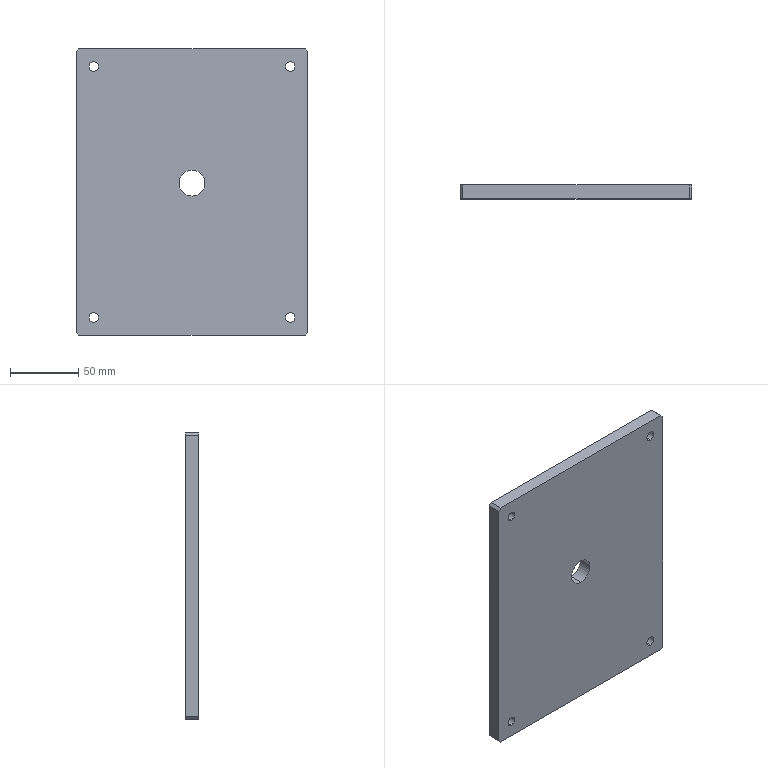Part | SolidWorks | features MirrorPattern 2, Chamfer 1, Cut 1, Extrusion 1, ICE 1 | 1 solid | 20 faces | box 170 x 10 x 210 mm | volume 352545 mm3 | cylinder 10 | plane 10 | commonest cylinder face diameters 7 x8 19 x2
STEP:
#1=CARTESIAN_POINT('',(-72.,10.,-95.5));
#2=VERTEX_POINT('',#1);
#3=CARTESIAN_POINT('',(-72.,10.,-88.5));
#4=VERTEX_POINT('',#3);
#5=CARTESIAN_POINT('',(-72.,10.,-92.));
#6=DIRECTION('',(0.,1.,0.));
#7=DIRECTION('',(0.,0.,-1.));
#8=AXIS2_PLACEMENT_3D('',#5,#6,#7);
#9=CIRCLE('',#8,3.5);
#10=EDGE_CURVE('',#2,#4,#9,.T.);
#11=ORIENTED_EDGE('',*,*,#10,.T.);
#12=CARTESIAN_POINT('',(-72.,0.,-88.5));
#13=VERTEX_POINT('',#12);
#14=CARTESIAN_POINT('',(-72.,10.001,-88.5));
#15=DIRECTION('',(0.,-1.,0.));
#16=VECTOR('',#15,1000.);
#17=LINE('',#14,#16);
#18=EDGE_CURVE('',#4,#13,#17,.T.);
#19=ORIENTED_EDGE('',*,*,#18,.T.);
#20=CARTESIAN_POINT('',(-72.,0.,-95.5));
#21=VERTEX_POINT('',#20);
#22=CARTESIAN_POINT('',(-72.,0.,-92.));
#23=DIRECTION('',(0.,-1.,0.));
#24=DIRECTION('',(0.,0.,1.));
#25=AXIS2_PLACEMENT_3D('',#22,#23,#24);
#26=CIRCLE('',#25,3.5);
#27=EDGE_CURVE('',#13,#21,#26,.T.);
#28=ORIENTED_EDGE('',*,*,#27,.T.);
#29=CARTESIAN_POINT('',(-72.,10.001,-95.5));
#30=DIRECTION('',(0.,-1.,0.));
#31=VECTOR('',#30,1000.);
#32=LINE('',#29,#31);
#33=EDGE_CURVE('',#2,#21,#32,.T.);
#34=ORIENTED_EDGE('',*,*,#33,.F.);
#35=EDGE_LOOP('',(#11,#19,#28,#34));
#36=FACE_OUTER_BOUND('',#35,.T.);
#37=CARTESIAN_POINT('',(-72.,10.001,-92.));
#38=DIRECTION('',(0.,-1.,0.));
#39=DIRECTION('',(0.,0.,-1.));
#40=AXIS2_PLACEMENT_3D('',#37,#38,#39);
#41=CYLINDRICAL_SURFACE('',#40,3.5);
#42=ADVANCED_FACE('',(#36),#41,.F.);
#43=CARTESIAN_POINT('',(72.,10.,-88.5));
#44=VERTEX_POINT('',#43);
#45=CARTESIAN_POINT('',(72.,10.,-95.5));
#46=VERTEX_POINT('',#45);
#47=CARTESIAN_POINT('',(72.,10.,-92.));
#48=DIRECTION('',(0.,-1.,0.));
#49=DIRECTION('',(0.,0.,-1.));
#50=AXIS2_PLACEMENT_3D('',#47,#48,#49);
#51=CIRCLE('',#50,3.5);
#52=EDGE_CURVE('',#44,#46,#51,.T.);
#53=ORIENTED_EDGE('',*,*,#52,.F.);
#54=CARTESIAN_POINT('',(72.,0.,-88.5));
#55=VERTEX_POINT('',#54);
#56=CARTESIAN_POINT('',(72.,10.001,-88.5));
#57=DIRECTION('',(0.,-1.,0.));
#58=VECTOR('',#57,1000.);
#59=LINE('',#56,#58);
#60=EDGE_CURVE('',#44,#55,#59,.T.);
#61=ORIENTED_EDGE('',*,*,#60,.T.);
#62=CARTESIAN_POINT('',(72.,0.,-95.5));
#63=VERTEX_POINT('',#62);
#64=CARTESIAN_POINT('',(72.,0.,-92.));
#65=DIRECTION('',(0.,1.,0.));
#66=DIRECTION('',(0.,0.,1.));
#67=AXIS2_PLACEMENT_3D('',#64,#65,#66);
#68=CIRCLE('',#67,3.5);
#69=EDGE_CURVE('',#63,#55,#68,.T.);
#70=ORIENTED_EDGE('',*,*,#69,.F.);
#71=CARTESIAN_POINT('',(72.,10.001,-95.5));
#72=DIRECTION('',(0.,-1.,0.));
#73=VECTOR('',#72,1000.);
#74=LINE('',#71,#73);
#75=EDGE_CURVE('',#46,#63,#74,.T.);
#76=ORIENTED_EDGE('',*,*,#75,.F.);
#77=EDGE_LOOP('',(#53,#61,#70,#76));
#78=FACE_OUTER_BOUND('',#77,.T.);
#79=CARTESIAN_POINT('',(72.,10.001,-92.));
#80=DIRECTION('',(0.,-1.,0.));
#81=DIRECTION('',(0.,0.,-1.));
#82=AXIS2_PLACEMENT_3D('',#79,#80,#81);
#83=CYLINDRICAL_SURFACE('',#82,3.5);
#84=ADVANCED_FACE('',(#78),#83,.F.);
#85=CARTESIAN_POINT('',(-72.,10.,95.5));
#86=VERTEX_POINT('',#85);
#87=CARTESIAN_POINT('',(-72.,10.,88.5));
#88=VERTEX_POINT('',#87);
#89=CARTESIAN_POINT('',(-72.,10.,92.));
#90=DIRECTION('',(0.,-1.,0.));
#91=DIRECTION('',(0.,0.,-1.));
#92=AXIS2_PLACEMENT_3D('',#89,#90,#91);
#93=CIRCLE('',#92,3.5);
#94=EDGE_CURVE('',#86,#88,#93,.T.);
#95=ORIENTED_EDGE('',*,*,#94,.F.);
#96=CARTESIAN_POINT('',(-72.,0.,95.5));
#97=VERTEX_POINT('',#96);
#98=CARTESIAN_POINT('',(-72.,10.001,95.5));
#99=DIRECTION('',(0.,-1.,0.));
#100=VECTOR('',#99,1000.);
#101=LINE('',#98,#100);
#102=EDGE_CURVE('',#86,#97,#101,.T.);
#103=ORIENTED_EDGE('',*,*,#102,.T.);
#104=CARTESIAN_POINT('',(-72.,0.,88.5));
#105=VERTEX_POINT('',#104);
#106=CARTESIAN_POINT('',(-72.,0.,92.));
#107=DIRECTION('',(0.,1.,0.));
#108=DIRECTION('',(0.,0.,-1.));
#109=AXIS2_PLACEMENT_3D('',#106,#107,#108);
#110=CIRCLE('',#109,3.5);
#111=EDGE_CURVE('',#105,#97,#110,.T.);
#112=ORIENTED_EDGE('',*,*,#111,.F.);
#113=CARTESIAN_POINT('',(-72.,10.001,88.5));
#114=DIRECTION('',(0.,-1.,0.));
#115=VECTOR('',#114,1000.);
#116=LINE('',#113,#115);
#117=EDGE_CURVE('',#88,#105,#116,.T.);
#118=ORIENTED_EDGE('',*,*,#117,.F.);
#119=EDGE_LOOP('',(#95,#103,#112,#118));
#120=FACE_OUTER_BOUND('',#119,.T.);
#121=CARTESIAN_POINT('',(-72.,10.001,92.));
#122=DIRECTION('',(0.,-1.,0.));
#123=DIRECTION('',(0.,0.,-1.));
#124=AXIS2_PLACEMENT_3D('',#121,#122,#123);
#125=CYLINDRICAL_SURFACE('',#124,3.5);
#126=ADVANCED_FACE('',(#120),#125,.F.);
#127=CARTESIAN_POINT('',(72.,10.,88.5));
#128=VERTEX_POINT('',#127);
#129=CARTESIAN_POINT('',(72.,10.,95.5));
#130=VERTEX_POINT('',#129);
#131=CARTESIAN_POINT('',(72.,10.,92.));
#132=DIRECTION('',(0.,1.,0.));
#133=DIRECTION('',(0.,0.,-1.));
#134=AXIS2_PLACEMENT_3D('',#131,#132,#133);
#135=CIRCLE('',#134,3.5);
#136=EDGE_CURVE('',#128,#130,#135,.T.);
#137=ORIENTED_EDGE('',*,*,#136,.T.);
#138=CARTESIAN_POINT('',(72.,0.,95.5));
#139=VERTEX_POINT('',#138);
#140=CARTESIAN_POINT('',(72.,10.001,95.5));
#141=DIRECTION('',(0.,-1.,0.));
#142=VECTOR('',#141,1000.);
#143=LINE('',#140,#142);
#144=EDGE_CURVE('',#130,#139,#143,.T.);
#145=ORIENTED_EDGE('',*,*,#144,.T.);
#146=CARTESIAN_POINT('',(72.,0.,88.5));
#147=VERTEX_POINT('',#146);
#148=CARTESIAN_POINT('',(72.,0.,92.));
#149=DIRECTION('',(0.,-1.,0.));
#150=DIRECTION('',(0.,0.,-1.));
#151=AXIS2_PLACEMENT_3D('',#148,#149,#150);
#152=CIRCLE('',#151,3.5);
#153=EDGE_CURVE('',#139,#147,#152,.T.);
#154=ORIENTED_EDGE('',*,*,#153,.T.);
#155=CARTESIAN_POINT('',(72.,10.001,88.5));
#156=DIRECTION('',(0.,-1.,0.));
#157=VECTOR('',#156,1000.);
#158=LINE('',#155,#157);
#159=EDGE_CURVE('',#128,#147,#158,.T.);
#160=ORIENTED_EDGE('',*,*,#159,.F.);
#161=EDGE_LOOP('',(#137,#145,#154,#160));
#162=FACE_OUTER_BOUND('',#161,.T.);
#163=CARTESIAN_POINT('',(72.,10.001,92.));
#164=DIRECTION('',(0.,-1.,0.));
#165=DIRECTION('',(0.,0.,-1.));
#166=AXIS2_PLACEMENT_3D('',#163,#164,#165);
#167=CYLINDRICAL_SURFACE('',#166,3.5);
#168=ADVANCED_FACE('',(#162),#167,.F.);
#169=CARTESIAN_POINT('',(0.,0.,-3.));
#170=VERTEX_POINT('',#169);
#171=CARTESIAN_POINT('',(0.,0.,16.));
#172=VERTEX_POINT('',#171);
#173=CARTESIAN_POINT('',(0.,0.,6.5));
#174=DIRECTION('',(0.,1.,0.));
#175=DIRECTION('',(0.,0.,-1.));
#176=AXIS2_PLACEMENT_3D('',#173,#174,#175);
#177=CIRCLE('',#176,9.5);
#178=EDGE_CURVE('',#170,#172,#177,.T.);
#179=ORIENTED_EDGE('',*,*,#178,.F.);
#180=CARTESIAN_POINT('',(0.,10.,-3.));
#181=VERTEX_POINT('',#180);
#182=CARTESIAN_POINT('',(0.,-0.001,-3.));
#183=DIRECTION('',(0.,1.,0.));
#184=VECTOR('',#183,1000.);
#185=LINE('',#182,#184);
#186=EDGE_CURVE('',#170,#181,#185,.T.);
#187=ORIENTED_EDGE('',*,*,#186,.T.);
#188=CARTESIAN_POINT('',(0.,10.,16.));
#189=VERTEX_POINT('',#188);
#190=CARTESIAN_POINT('',(0.,10.,6.5));
#191=DIRECTION('',(0.,1.,0.));
#192=DIRECTION('',(0.,0.,1.));
#193=AXIS2_PLACEMENT_3D('',#190,#191,#192);
#194=CIRCLE('',#193,9.5);
#195=EDGE_CURVE('',#181,#189,#194,.T.);
#196=ORIENTED_EDGE('',*,*,#195,.T.);
#197=CARTESIAN_POINT('',(0.,-0.001,16.));
#198=DIRECTION('',(0.,1.,0.));
#199=VECTOR('',#198,1000.);
#200=LINE('',#197,#199);
#201=EDGE_CURVE('',#172,#189,#200,.T.);
#202=ORIENTED_EDGE('',*,*,#201,.F.);
#203=EDGE_LOOP('',(#179,#187,#196,#202));
#204=FACE_OUTER_BOUND('',#203,.T.);
#205=CARTESIAN_POINT('',(0.,-0.001,6.5));
#206=DIRECTION('',(0.,1.,0.));
#207=DIRECTION('',(0.,0.,1.));
#208=AXIS2_PLACEMENT_3D('',#205,#206,#207);
#209=CYLINDRICAL_SURFACE('',#208,9.5);
#210=ADVANCED_FACE('',(#204),#209,.F.);
#211=CARTESIAN_POINT('',(85.,0.,103.));
#212=VERTEX_POINT('',#211);
#213=CARTESIAN_POINT('',(85.,0.,-103.));
#214=VERTEX_POINT('',#213);
#215=CARTESIAN_POINT('',(85.,0.,105.));
#216=DIRECTION('',(0.,0.,-1.));
#217=VECTOR('',#216,1000.);
#218=LINE('',#215,#217);
#219=EDGE_CURVE('',#212,#214,#218,.T.);
#220=ORIENTED_EDGE('',*,*,#219,.T.);
#221=CARTESIAN_POINT('',(85.,10.,-103.));
#222=VERTEX_POINT('',#221);
#223=CARTESIAN_POINT('',(85.,10.,-103.));
#224=DIRECTION('',(0.,1.,0.));
#225=VECTOR('',#224,1000.);
#226=LINE('',#223,#225);
#227=EDGE_CURVE('',#214,#222,#226,.T.);
#228=ORIENTED_EDGE('',*,*,#227,.T.);
#229=CARTESIAN_POINT('',(85.,10.,103.));
#230=VERTEX_POINT('',#229);
#231=CARTESIAN_POINT('',(85.,10.,105.));
#232=DIRECTION('',(0.,0.,-1.));
#233=VECTOR('',#232,1000.);
#234=LINE('',#231,#233);
#235=EDGE_CURVE('',#230,#222,#234,.T.);
#236=ORIENTED_EDGE('',*,*,#235,.F.);
#237=CARTESIAN_POINT('',(85.,10.,103.));
#238=DIRECTION('',(0.,-1.,0.));
#239=VECTOR('',#238,1000.);
#240=LINE('',#237,#239);
#241=EDGE_CURVE('',#230,#212,#240,.T.);
#242=ORIENTED_EDGE('',*,*,#241,.T.);
#243=EDGE_LOOP('',(#220,#228,#236,#242));
#244=FACE_OUTER_BOUND('',#243,.T.);
#245=CARTESIAN_POINT('',(85.,10.,105.));
#246=DIRECTION('',(-1.,0.,0.));
#247=DIRECTION('',(0.,0.,1.));
#248=AXIS2_PLACEMENT_3D('',#245,#246,#247);
#249=PLANE('',#248);
#250=ADVANCED_FACE('',(#244),#249,.F.);
#251=CARTESIAN_POINT('',(83.,0.,-105.));
#252=VERTEX_POINT('',#251);
#253=CARTESIAN_POINT('',(-83.,0.,-105.));
#254=VERTEX_POINT('',#253);
#255=CARTESIAN_POINT('',(-85.,0.,-105.));
#256=DIRECTION('',(-1.,0.,0.));
#257=VECTOR('',#256,1000.);
#258=LINE('',#255,#257);
#259=EDGE_CURVE('',#252,#254,#258,.T.);
#260=ORIENTED_EDGE('',*,*,#259,.T.);
#261=CARTESIAN_POINT('',(-83.,10.,-105.));
#262=VERTEX_POINT('',#261);
#263=CARTESIAN_POINT('',(-83.,10.,-105.));
#264=DIRECTION('',(0.,1.,0.));
#265=VECTOR('',#264,1000.);
#266=LINE('',#263,#265);
#267=EDGE_CURVE('',#254,#262,#266,.T.);
#268=ORIENTED_EDGE('',*,*,#267,.T.);
#269=CARTESIAN_POINT('',(83.,10.,-105.));
#270=VERTEX_POINT('',#269);
#271=CARTESIAN_POINT('',(-85.,10.,-105.));
#272=DIRECTION('',(-1.,0.,0.));
#273=VECTOR('',#272,1000.);
#274=LINE('',#271,#273);
#275=EDGE_CURVE('',#270,#262,#274,.T.);
#276=ORIENTED_EDGE('',*,*,#275,.F.);
#277=CARTESIAN_POINT('',(83.,10.,-105.));
#278=DIRECTION('',(0.,-1.,0.));
#279=VECTOR('',#278,1000.);
#280=LINE('',#277,#279);
#281=EDGE_CURVE('',#270,#252,#280,.T.);
#282=ORIENTED_EDGE('',*,*,#281,.T.);
#283=EDGE_LOOP('',(#260,#268,#276,#282));
#284=FACE_OUTER_BOUND('',#283,.T.);
#285=CARTESIAN_POINT('',(-85.,10.,-105.));
#286=DIRECTION('',(0.,0.,1.));
#287=DIRECTION('',(1.,0.,0.));
#288=AXIS2_PLACEMENT_3D('',#285,#286,#287);
#289=PLANE('',#288);
#290=ADVANCED_FACE('',(#284),#289,.F.);
#291=CARTESIAN_POINT('',(-85.,0.,-103.));
#292=VERTEX_POINT('',#291);
#293=CARTESIAN_POINT('',(-85.,0.,103.));
#294=VERTEX_POINT('',#293);
#295=CARTESIAN_POINT('',(-85.,0.,105.));
#296=DIRECTION('',(0.,0.,1.));
#297=VECTOR('',#296,1000.);
#298=LINE('',#295,#297);
#299=EDGE_CURVE('',#292,#294,#298,.T.);
#300=ORIENTED_EDGE('',*,*,#299,.T.);
#301=CARTESIAN_POINT('',(-85.,10.,103.));
#302=VERTEX_POINT('',#301);
#303=CARTESIAN_POINT('',(-85.,10.,103.));
#304=DIRECTION('',(0.,1.,0.));
#305=VECTOR('',#304,1000.);
#306=LINE('',#303,#305);
#307=EDGE_CURVE('',#294,#302,#306,.T.);
#308=ORIENTED_EDGE('',*,*,#307,.T.);
#309=CARTESIAN_POINT('',(-85.,10.,-103.));
#310=VERTEX_POINT('',#309);
#311=CARTESIAN_POINT('',(-85.,10.,105.));
#312=DIRECTION('',(0.,0.,1.));
#313=VECTOR('',#312,1000.);
#314=LINE('',#311,#313);
#315=EDGE_CURVE('',#310,#302,#314,.T.);
#316=ORIENTED_EDGE('',*,*,#315,.F.);
#317=CARTESIAN_POINT('',(-85.,10.,-103.));
#318=DIRECTION('',(0.,-1.,0.));
#319=VECTOR('',#318,1000.);
#320=LINE('',#317,#319);
#321=EDGE_CURVE('',#310,#292,#320,.T.);
#322=ORIENTED_EDGE('',*,*,#321,.T.);
#323=EDGE_LOOP('',(#300,#308,#316,#322));
#324=FACE_OUTER_BOUND('',#323,.T.);
#325=CARTESIAN_POINT('',(-85.,10.,105.));
#326=DIRECTION('',(1.,0.,0.));
#327=DIRECTION('',(0.,0.,-1.));
#328=AXIS2_PLACEMENT_3D('',#325,#326,#327);
#329=PLANE('',#328);
#330=ADVANCED_FACE('',(#324),#329,.F.);
#331=CARTESIAN_POINT('',(-83.,10.,105.));
#332=VERTEX_POINT('',#331);
#333=CARTESIAN_POINT('',(83.,10.,105.));
#334=VERTEX_POINT('',#333);
#335=CARTESIAN_POINT('',(-85.,10.,105.));
#336=DIRECTION('',(1.,0.,0.));
#337=VECTOR('',#336,1000.);
#338=LINE('',#335,#337);
#339=EDGE_CURVE('',#332,#334,#338,.T.);
#340=ORIENTED_EDGE('',*,*,#339,.F.);
#341=CARTESIAN_POINT('',(-83.,0.,105.));
#342=VERTEX_POINT('',#341);
#343=CARTESIAN_POINT('',(-83.,10.,105.));
#344=DIRECTION('',(0.,-1.,0.));
#345=VECTOR('',#344,1000.);
#346=LINE('',#343,#345);
#347=EDGE_CURVE('',#332,#342,#346,.T.);
#348=ORIENTED_EDGE('',*,*,#347,.T.);
#349=CARTESIAN_POINT('',(83.,0.,105.));
#350=VERTEX_POINT('',#349);
#351=CARTESIAN_POINT('',(-85.,0.,105.));
#352=DIRECTION('',(1.,0.,0.));
#353=VECTOR('',#352,1000.);
#354=LINE('',#351,#353);
#355=EDGE_CURVE('',#342,#350,#354,.T.);
#356=ORIENTED_EDGE('',*,*,#355,.T.);
#357=CARTESIAN_POINT('',(83.,10.,105.));
#358=DIRECTION('',(0.,1.,0.));
#359=VECTOR('',#358,1000.);
#360=LINE('',#357,#359);
#361=EDGE_CURVE('',#350,#334,#360,.T.);
#362=ORIENTED_EDGE('',*,*,#361,.T.);
#363=EDGE_LOOP('',(#340,#348,#356,#362));
#364=FACE_OUTER_BOUND('',#363,.T.);
#365=CARTESIAN_POINT('',(-85.,10.,105.));
#366=DIRECTION('',(0.,0.,-1.));
#367=DIRECTION('',(-1.,0.,0.));
#368=AXIS2_PLACEMENT_3D('',#365,#366,#367);
#369=PLANE('',#368);
#370=ADVANCED_FACE('',(#364),#369,.F.);
#371=ORIENTED_EDGE('',*,*,#10,.F.);
#372=CARTESIAN_POINT('',(-72.,10.,-92.));
#373=DIRECTION('',(0.,1.,0.));
#374=DIRECTION('',(0.,0.,-1.));
#375=AXIS2_PLACEMENT_3D('',#372,#373,#374);
#376=CIRCLE('',#375,3.5);
#377=EDGE_CURVE('',#4,#2,#376,.T.);
#378=ORIENTED_EDGE('',*,*,#377,.F.);
#379=EDGE_LOOP('',(#371,#378));
#380=FACE_BOUND('',#379,.T.);
#381=CARTESIAN_POINT('',(72.,10.,-92.));
#382=DIRECTION('',(0.,-1.,0.));
#383=DIRECTION('',(0.,0.,-1.));
#384=AXIS2_PLACEMENT_3D('',#381,#382,#383);
#385=CIRCLE('',#384,3.5);
#386=EDGE_CURVE('',#46,#44,#385,.T.);
#387=ORIENTED_EDGE('',*,*,#386,.T.);
#388=ORIENTED_EDGE('',*,*,#52,.T.);
#389=EDGE_LOOP('',(#387,#388));
#390=FACE_BOUND('',#389,.T.);
#391=CARTESIAN_POINT('',(-72.,10.,92.));
#392=DIRECTION('',(0.,-1.,0.));
#393=DIRECTION('',(0.,0.,-1.));
#394=AXIS2_PLACEMENT_3D('',#391,#392,#393);
#395=CIRCLE('',#394,3.5);
#396=EDGE_CURVE('',#88,#86,#395,.T.);
#397=ORIENTED_EDGE('',*,*,#396,.T.);
#398=ORIENTED_EDGE('',*,*,#94,.T.);
#399=EDGE_LOOP('',(#397,#398));
#400=FACE_BOUND('',#399,.T.);
#401=ORIENTED_EDGE('',*,*,#136,.F.);
#402=CARTESIAN_POINT('',(72.,10.,92.));
#403=DIRECTION('',(0.,1.,0.));
#404=DIRECTION('',(0.,0.,-1.));
#405=AXIS2_PLACEMENT_3D('',#402,#403,#404);
#406=CIRCLE('',#405,3.5);
#407=EDGE_CURVE('',#130,#128,#406,.T.);
#408=ORIENTED_EDGE('',*,*,#407,.F.);
#409=EDGE_LOOP('',(#401,#408));
#410=FACE_BOUND('',#409,.T.);
#411=CARTESIAN_POINT('',(0.,10.,6.5));
#412=DIRECTION('',(0.,1.,0.));
#413=DIRECTION('',(0.,0.,1.));
#414=AXIS2_PLACEMENT_3D('',#411,#412,#413);
#415=CIRCLE('',#414,9.5);
#416=EDGE_CURVE('',#189,#181,#415,.T.);
#417=ORIENTED_EDGE('',*,*,#416,.F.);
#418=ORIENTED_EDGE('',*,*,#195,.F.);
#419=EDGE_LOOP('',(#417,#418));
#420=FACE_BOUND('',#419,.T.);
#421=ORIENTED_EDGE('',*,*,#315,.T.);
#422=CARTESIAN_POINT('',(-83.,10.,105.));
#423=DIRECTION('',(0.7071,0.,0.7071));
#424=VECTOR('',#423,1000.);
#425=LINE('',#422,#424);
#426=EDGE_CURVE('',#302,#332,#425,.T.);
#427=ORIENTED_EDGE('',*,*,#426,.T.);
#428=ORIENTED_EDGE('',*,*,#339,.T.);
#429=CARTESIAN_POINT('',(85.,10.,103.));
#430=DIRECTION('',(0.7071,0.,-0.7071));
#431=VECTOR('',#430,1000.);
#432=LINE('',#429,#431);
#433=EDGE_CURVE('',#334,#230,#432,.T.);
#434=ORIENTED_EDGE('',*,*,#433,.T.);
#435=ORIENTED_EDGE('',*,*,#235,.T.);
#436=CARTESIAN_POINT('',(83.,10.,-105.));
#437=DIRECTION('',(-0.7071,0.,-0.7071));
#438=VECTOR('',#437,1000.);
#439=LINE('',#436,#438);
#440=EDGE_CURVE('',#222,#270,#439,.T.);
#441=ORIENTED_EDGE('',*,*,#440,.T.);
#442=ORIENTED_EDGE('',*,*,#275,.T.);
#443=CARTESIAN_POINT('',(-85.,10.,-103.));
#444=DIRECTION('',(-0.7071,0.,0.7071));
#445=VECTOR('',#444,1000.);
#446=LINE('',#443,#445);
#447=EDGE_CURVE('',#262,#310,#446,.T.);
#448=ORIENTED_EDGE('',*,*,#447,.T.);
#449=EDGE_LOOP('',(#421,#427,#428,#434,#435,#441,#442,#448));
#450=FACE_OUTER_BOUND('',#449,.T.);
#451=CARTESIAN_POINT('',(0.,10.,0.));
#452=DIRECTION('',(0.,-1.,0.));
#453=DIRECTION('',(0.,0.,-1.));
#454=AXIS2_PLACEMENT_3D('',#451,#452,#453);
#455=PLANE('',#454);
#456=ADVANCED_FACE('',(#380,#390,#400,#410,#420,#450),#455,.F.);
#457=CARTESIAN_POINT('',(-72.,0.,-92.));
#458=DIRECTION('',(0.,-1.,0.));
#459=DIRECTION('',(0.,0.,1.));
#460=AXIS2_PLACEMENT_3D('',#457,#458,#459);
#461=CIRCLE('',#460,3.5);
#462=EDGE_CURVE('',#21,#13,#461,.T.);
#463=ORIENTED_EDGE('',*,*,#462,.F.);
#464=ORIENTED_EDGE('',*,*,#27,.F.);
#465=EDGE_LOOP('',(#463,#464));
#466=FACE_BOUND('',#465,.T.);
#467=ORIENTED_EDGE('',*,*,#69,.T.);
#468=CARTESIAN_POINT('',(72.,0.,-92.));
#469=DIRECTION('',(0.,1.,0.));
#470=DIRECTION('',(0.,0.,1.));
#471=AXIS2_PLACEMENT_3D('',#468,#469,#470);
#472=CIRCLE('',#471,3.5);
#473=EDGE_CURVE('',#55,#63,#472,.T.);
#474=ORIENTED_EDGE('',*,*,#473,.T.);
#475=EDGE_LOOP('',(#467,#474));
#476=FACE_BOUND('',#475,.T.);
#477=ORIENTED_EDGE('',*,*,#111,.T.);
#478=CARTESIAN_POINT('',(-72.,0.,92.));
#479=DIRECTION('',(0.,1.,0.));
#480=DIRECTION('',(0.,0.,-1.));
#481=AXIS2_PLACEMENT_3D('',#478,#479,#480);
#482=CIRCLE('',#481,3.5);
#483=EDGE_CURVE('',#97,#105,#482,.T.);
#484=ORIENTED_EDGE('',*,*,#483,.T.);
#485=EDGE_LOOP('',(#477,#484));
#486=FACE_BOUND('',#485,.T.);
#487=CARTESIAN_POINT('',(72.,0.,92.));
#488=DIRECTION('',(0.,-1.,0.));
#489=DIRECTION('',(0.,0.,-1.));
#490=AXIS2_PLACEMENT_3D('',#487,#488,#489);
#491=CIRCLE('',#490,3.5);
#492=EDGE_CURVE('',#147,#139,#491,.T.);
#493=ORIENTED_EDGE('',*,*,#492,.F.);
#494=ORIENTED_EDGE('',*,*,#153,.F.);
#495=EDGE_LOOP('',(#493,#494));
#496=FACE_BOUND('',#495,.T.);
#497=CARTESIAN_POINT('',(0.,0.,6.5));
#498=DIRECTION('',(0.,1.,0.));
#499=DIRECTION('',(0.,0.,-1.));
#500=AXIS2_PLACEMENT_3D('',#497,#498,#499);
#501=CIRCLE('',#500,9.5);
#502=EDGE_CURVE('',#172,#170,#501,.T.);
#503=ORIENTED_EDGE('',*,*,#502,.T.);
#504=ORIENTED_EDGE('',*,*,#178,.T.);
#505=EDGE_LOOP('',(#503,#504));
#506=FACE_BOUND('',#505,.T.);
#507=ORIENTED_EDGE('',*,*,#355,.F.);
#508=CARTESIAN_POINT('',(-94.,0.,94.));
#509=DIRECTION('',(-0.7071,0.,-0.7071));
#510=VECTOR('',#509,1000.);
#511=LINE('',#508,#510);
#512=EDGE_CURVE('',#342,#294,#511,.T.);
#513=ORIENTED_EDGE('',*,*,#512,.T.);
#514=ORIENTED_EDGE('',*,*,#299,.F.);
#515=CARTESIAN_POINT('',(-94.,0.,-94.));
#516=DIRECTION('',(0.7071,0.,-0.7071));
#517=VECTOR('',#516,1000.);
#518=LINE('',#515,#517);
#519=EDGE_CURVE('',#292,#254,#518,.T.);
#520=ORIENTED_EDGE('',*,*,#519,.T.);
#521=ORIENTED_EDGE('',*,*,#259,.F.);
#522=CARTESIAN_POINT('',(94.,0.,-94.));
#523=DIRECTION('',(0.7071,0.,0.7071));
#524=VECTOR('',#523,1000.);
#525=LINE('',#522,#524);
#526=EDGE_CURVE('',#252,#214,#525,.T.);
#527=ORIENTED_EDGE('',*,*,#526,.T.);
#528=ORIENTED_EDGE('',*,*,#219,.F.);
#529=CARTESIAN_POINT('',(94.,0.,94.));
#530=DIRECTION('',(-0.7071,0.,0.7071));
#531=VECTOR('',#530,1000.);
#532=LINE('',#529,#531);
#533=EDGE_CURVE('',#212,#350,#532,.T.);
#534=ORIENTED_EDGE('',*,*,#533,.T.);
#535=EDGE_LOOP('',(#507,#513,#514,#520,#521,#527,#528,#534));
#536=FACE_OUTER_BOUND('',#535,.T.);
#537=CARTESIAN_POINT('',(0.,0.,0.));
#538=DIRECTION('',(0.,-1.,0.));
#539=DIRECTION('',(0.,0.,-1.));
#540=AXIS2_PLACEMENT_3D('',#537,#538,#539);
#541=PLANE('',#540);
#542=ADVANCED_FACE('',(#466,#476,#486,#496,#506,#536),#541,.T.);
#543=ORIENTED_EDGE('',*,*,#186,.F.);
#544=ORIENTED_EDGE('',*,*,#502,.F.);
#545=ORIENTED_EDGE('',*,*,#201,.T.);
#546=ORIENTED_EDGE('',*,*,#416,.T.);
#547=EDGE_LOOP('',(#543,#544,#545,#546));
#548=FACE_OUTER_BOUND('',#547,.T.);
#549=CARTESIAN_POINT('',(0.,-0.001,6.5));
#550=DIRECTION('',(0.,1.,0.));
#551=DIRECTION('',(0.,0.,1.));
#552=AXIS2_PLACEMENT_3D('',#549,#550,#551);
#553=CYLINDRICAL_SURFACE('',#552,9.5);
#554=ADVANCED_FACE('',(#548),#553,.F.);
#555=ORIENTED_EDGE('',*,*,#144,.F.);
#556=ORIENTED_EDGE('',*,*,#407,.T.);
#557=ORIENTED_EDGE('',*,*,#159,.T.);
#558=ORIENTED_EDGE('',*,*,#492,.T.);
#559=EDGE_LOOP('',(#555,#556,#557,#558));
#560=FACE_OUTER_BOUND('',#559,.T.);
#561=CARTESIAN_POINT('',(72.,10.001,92.));
#562=DIRECTION('',(0.,-1.,0.));
#563=DIRECTION('',(0.,0.,-1.));
#564=AXIS2_PLACEMENT_3D('',#561,#562,#563);
#565=CYLINDRICAL_SURFACE('',#564,3.5);
#566=ADVANCED_FACE('',(#560),#565,.F.);
#567=ORIENTED_EDGE('',*,*,#102,.F.);
#568=ORIENTED_EDGE('',*,*,#396,.F.);
#569=ORIENTED_EDGE('',*,*,#117,.T.);
#570=ORIENTED_EDGE('',*,*,#483,.F.);
#571=EDGE_LOOP('',(#567,#568,#569,#570));
#572=FACE_OUTER_BOUND('',#571,.T.);
#573=CARTESIAN_POINT('',(-72.,10.001,92.));
#574=DIRECTION('',(0.,-1.,0.));
#575=DIRECTION('',(0.,0.,-1.));
#576=AXIS2_PLACEMENT_3D('',#573,#574,#575);
#577=CYLINDRICAL_SURFACE('',#576,3.5);
#578=ADVANCED_FACE('',(#572),#577,.F.);
#579=ORIENTED_EDGE('',*,*,#60,.F.);
#580=ORIENTED_EDGE('',*,*,#386,.F.);
#581=ORIENTED_EDGE('',*,*,#75,.T.);
#582=ORIENTED_EDGE('',*,*,#473,.F.);
#583=EDGE_LOOP('',(#579,#580,#581,#582));
#584=FACE_OUTER_BOUND('',#583,.T.);
#585=CARTESIAN_POINT('',(72.,10.001,-92.));
#586=DIRECTION('',(0.,-1.,0.));
#587=DIRECTION('',(0.,0.,-1.));
#588=AXIS2_PLACEMENT_3D('',#585,#586,#587);
#589=CYLINDRICAL_SURFACE('',#588,3.5);
#590=ADVANCED_FACE('',(#584),#589,.F.);
#591=ORIENTED_EDGE('',*,*,#18,.F.);
#592=ORIENTED_EDGE('',*,*,#377,.T.);
#593=ORIENTED_EDGE('',*,*,#33,.T.);
#594=ORIENTED_EDGE('',*,*,#462,.T.);
#595=EDGE_LOOP('',(#591,#592,#593,#594));
#596=FACE_OUTER_BOUND('',#595,.T.);
#597=CARTESIAN_POINT('',(-72.,10.001,-92.));
#598=DIRECTION('',(0.,-1.,0.));
#599=DIRECTION('',(0.,0.,-1.));
#600=AXIS2_PLACEMENT_3D('',#597,#598,#599);
#601=CYLINDRICAL_SURFACE('',#600,3.5);
#602=ADVANCED_FACE('',(#596),#601,.F.);
#603=ORIENTED_EDGE('',*,*,#426,.F.);
#604=ORIENTED_EDGE('',*,*,#307,.F.);
#605=ORIENTED_EDGE('',*,*,#512,.F.);
#606=ORIENTED_EDGE('',*,*,#347,.F.);
#607=EDGE_LOOP('',(#603,#604,#605,#606));
#608=FACE_OUTER_BOUND('',#607,.T.);
#609=CARTESIAN_POINT('',(-83.,10.,105.));
#610=DIRECTION('',(0.7071,0.,-0.7071));
#611=DIRECTION('',(0.,-1.,0.));
#612=AXIS2_PLACEMENT_3D('',#609,#610,#611);
#613=PLANE('',#612);
#614=ADVANCED_FACE('',(#608),#613,.F.);
#615=ORIENTED_EDGE('',*,*,#447,.F.);
#616=ORIENTED_EDGE('',*,*,#267,.F.);
#617=ORIENTED_EDGE('',*,*,#519,.F.);
#618=ORIENTED_EDGE('',*,*,#321,.F.);
#619=EDGE_LOOP('',(#615,#616,#617,#618));
#620=FACE_OUTER_BOUND('',#619,.T.);
#621=CARTESIAN_POINT('',(-85.,10.,-103.));
#622=DIRECTION('',(0.7071,0.,0.7071));
#623=DIRECTION('',(0.,-1.,0.));
#624=AXIS2_PLACEMENT_3D('',#621,#622,#623);
#625=PLANE('',#624);
#626=ADVANCED_FACE('',(#620),#625,.F.);
#627=ORIENTED_EDGE('',*,*,#440,.F.);
#628=ORIENTED_EDGE('',*,*,#227,.F.);
#629=ORIENTED_EDGE('',*,*,#526,.F.);
#630=ORIENTED_EDGE('',*,*,#281,.F.);
#631=EDGE_LOOP('',(#627,#628,#629,#630));
#632=FACE_OUTER_BOUND('',#631,.T.);
#633=CARTESIAN_POINT('',(83.,10.,-105.));
#634=DIRECTION('',(-0.7071,0.,0.7071));
#635=DIRECTION('',(0.,-1.,0.));
#636=AXIS2_PLACEMENT_3D('',#633,#634,#635);
#637=PLANE('',#636);
#638=ADVANCED_FACE('',(#632),#637,.F.);
#639=ORIENTED_EDGE('',*,*,#433,.F.);
#640=ORIENTED_EDGE('',*,*,#361,.F.);
#641=ORIENTED_EDGE('',*,*,#533,.F.);
#642=ORIENTED_EDGE('',*,*,#241,.F.);
#643=EDGE_LOOP('',(#639,#640,#641,#642));
#644=FACE_OUTER_BOUND('',#643,.T.);
#645=CARTESIAN_POINT('',(85.,10.,103.));
#646=DIRECTION('',(-0.7071,0.,-0.7071));
#647=DIRECTION('',(0.,-1.,0.));
#648=AXIS2_PLACEMENT_3D('',#645,#646,#647);
#649=PLANE('',#648);
#650=ADVANCED_FACE('',(#644),#649,.F.);
#651=CLOSED_SHELL('',(#42,#84,#126,#168,#210,#250,#290,#330,#370,#456,#542,#554,#566,#578,#590,#602,#614,#626,#638,#650));
#652=MANIFOLD_SOLID_BREP('',#651);
#653=CARTESIAN_POINT('',(0.,0.,0.));
#654=DIRECTION('',(0.,0.,1.));
#655=DIRECTION('',(1.,0.,0.));
#656=AXIS2_PLACEMENT_3D('',#653,#654,#655);
#657=(LENGTH_UNIT()NAMED_UNIT(*)SI_UNIT(.MILLI.,.METRE.));
#658=UNCERTAINTY_MEASURE_WITH_UNIT(LENGTH_MEASURE(0.00001),#657,'','');
#659=(NAMED_UNIT(*)PLANE_ANGLE_UNIT()SI_UNIT($,.RADIAN.));
#660=(NAMED_UNIT(*)SI_UNIT($,.STERADIAN.)SOLID_ANGLE_UNIT());
#661=(GEOMETRIC_REPRESENTATION_CONTEXT(3)GLOBAL_UNCERTAINTY_ASSIGNED_CONTEXT((#658))GLOBAL_UNIT_ASSIGNED_CONTEXT((#657,#659,#660))REPRESENTATION_CONTEXT('',''));
#662=ADVANCED_BREP_SHAPE_REPRESENTATION('',(#652,#656),#661);